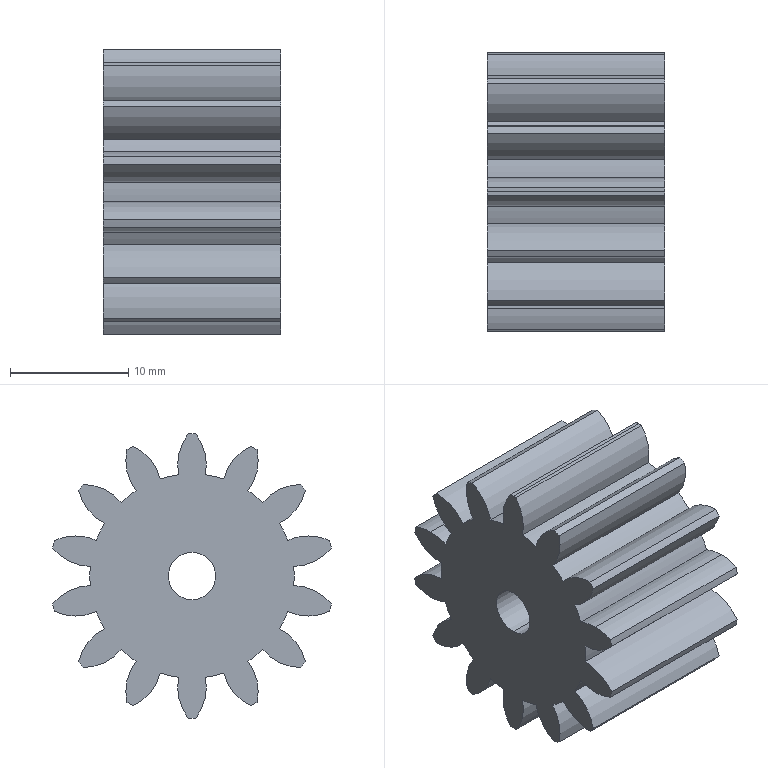Part | SolidWorks | features Boss 3, Cut 3, CirPattern 2, Fillet 2, Revolution 1 | 1 solid | 63 faces | box 15 x 23.532 x 24 mm | volume 4730 mm3 | cylinder 61 | plane 2 | commonest cylinder face diameters 8.4 x30 24 x15 17.248 x14 4 x2